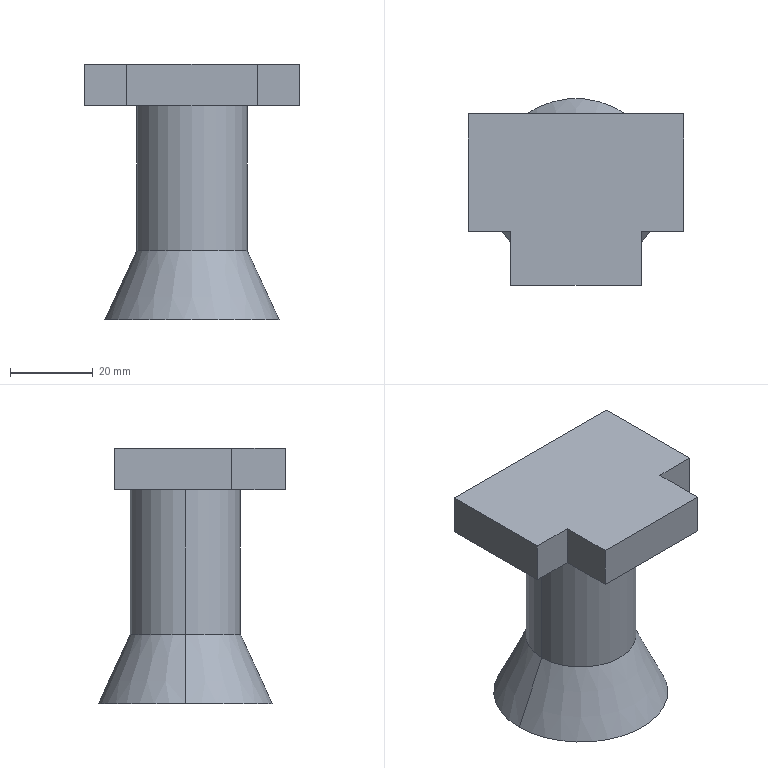Part | SolidWorks | features Extrusion 1, ICE 1, Revolution 1 | 1 solid | 15 faces | box 51.992 x 45.152 x 61.712 mm | volume 54023 mm3 | plane 11 | cone 2 | cylinder 2 | commonest cylinder face diameters 26.601 x2
STEP:
#1=CARTESIAN_POINT('',(-13.301,24.131,-45.));
#2=VERTEX_POINT('',#1);
#3=CARTESIAN_POINT('',(13.301,24.131,-45.));
#4=VERTEX_POINT('',#3);
#5=CARTESIAN_POINT('',(0.,24.131,-45.));
#6=DIRECTION('',(0.,0.,-1.));
#7=DIRECTION('',(-1.,0.,0.));
#8=AXIS2_PLACEMENT_3D('',#5,#6,#7);
#9=CIRCLE('',#8,13.301);
#10=EDGE_CURVE('',#2,#4,#9,.T.);
#11=ORIENTED_EDGE('',*,*,#10,.T.);
#12=CARTESIAN_POINT('',(21.021,24.131,-61.712));
#13=VERTEX_POINT('',#12);
#14=CARTESIAN_POINT('',(21.021,24.131,-61.712));
#15=DIRECTION('',(0.4194,0.,-0.9078));
#16=VECTOR('',#15,1000.);
#17=LINE('',#14,#16);
#18=EDGE_CURVE('',#4,#13,#17,.T.);
#19=ORIENTED_EDGE('',*,*,#18,.T.);
#20=CARTESIAN_POINT('',(-21.021,24.131,-61.712));
#21=VERTEX_POINT('',#20);
#22=CARTESIAN_POINT('',(0.,24.131,-61.712));
#23=DIRECTION('',(0.,0.,1.));
#24=DIRECTION('',(1.,0.,0.));
#25=AXIS2_PLACEMENT_3D('',#22,#23,#24);
#26=CIRCLE('',#25,21.021);
#27=EDGE_CURVE('',#13,#21,#26,.T.);
#28=ORIENTED_EDGE('',*,*,#27,.T.);
#29=CARTESIAN_POINT('',(-21.021,24.131,-61.712));
#30=DIRECTION('',(-0.4194,0.,-0.9078));
#31=VECTOR('',#30,1000.);
#32=LINE('',#29,#31);
#33=EDGE_CURVE('',#2,#21,#32,.T.);
#34=ORIENTED_EDGE('',*,*,#33,.F.);
#35=EDGE_LOOP('',(#11,#19,#28,#34));
#36=FACE_OUTER_BOUND('',#35,.T.);
#37=CARTESIAN_POINT('',(0.,24.131,-61.712));
#38=DIRECTION('',(0.,0.,-1.));
#39=DIRECTION('',(-1.,0.,0.));
#40=AXIS2_PLACEMENT_3D('',#37,#38,#39);
#41=CONICAL_SURFACE('',#40,21.021,0.4328);
#42=ADVANCED_FACE('',(#36),#41,.T.);
#43=ORIENTED_EDGE('',*,*,#10,.F.);
#44=CARTESIAN_POINT('',(-13.301,24.131,-10.));
#45=VERTEX_POINT('',#44);
#46=CARTESIAN_POINT('',(-13.301,24.131,-45.));
#47=DIRECTION('',(0.,0.,1.));
#48=VECTOR('',#47,1000.);
#49=LINE('',#46,#48);
#50=EDGE_CURVE('',#2,#45,#49,.T.);
#51=ORIENTED_EDGE('',*,*,#50,.T.);
#52=CARTESIAN_POINT('',(13.301,24.131,-10.));
#53=VERTEX_POINT('',#52);
#54=CARTESIAN_POINT('',(0.,24.131,-10.));
#55=DIRECTION('',(0.,0.,-1.));
#56=DIRECTION('',(1.,0.,0.));
#57=AXIS2_PLACEMENT_3D('',#54,#55,#56);
#58=CIRCLE('',#57,13.301);
#59=EDGE_CURVE('',#45,#53,#58,.T.);
#60=ORIENTED_EDGE('',*,*,#59,.T.);
#61=CARTESIAN_POINT('',(13.301,24.131,-45.));
#62=DIRECTION('',(0.,0.,1.));
#63=VECTOR('',#62,1000.);
#64=LINE('',#61,#63);
#65=EDGE_CURVE('',#4,#53,#64,.T.);
#66=ORIENTED_EDGE('',*,*,#65,.F.);
#67=EDGE_LOOP('',(#43,#51,#60,#66));
#68=FACE_OUTER_BOUND('',#67,.T.);
#69=CARTESIAN_POINT('',(0.,24.131,-45.));
#70=DIRECTION('',(0.,0.,1.));
#71=DIRECTION('',(1.,0.,0.));
#72=AXIS2_PLACEMENT_3D('',#69,#70,#71);
#73=CYLINDRICAL_SURFACE('',#72,13.301);
#74=ADVANCED_FACE('',(#68),#73,.T.);
#75=CARTESIAN_POINT('',(15.792,12.933,0.));
#76=VERTEX_POINT('',#75);
#77=CARTESIAN_POINT('',(25.996,12.933,0.));
#78=VERTEX_POINT('',#77);
#79=CARTESIAN_POINT('',(15.792,12.933,0.));
#80=DIRECTION('',(1.,0.,0.));
#81=VECTOR('',#80,1000.);
#82=LINE('',#79,#81);
#83=EDGE_CURVE('',#76,#78,#82,.T.);
#84=ORIENTED_EDGE('',*,*,#83,.F.);
#85=CARTESIAN_POINT('',(15.792,12.933,-10.));
#86=VERTEX_POINT('',#85);
#87=CARTESIAN_POINT('',(15.792,12.933,-10.));
#88=DIRECTION('',(0.,0.,1.));
#89=VECTOR('',#88,1000.);
#90=LINE('',#87,#89);
#91=EDGE_CURVE('',#86,#76,#90,.T.);
#92=ORIENTED_EDGE('',*,*,#91,.F.);
#93=CARTESIAN_POINT('',(25.996,12.933,-10.));
#94=VERTEX_POINT('',#93);
#95=CARTESIAN_POINT('',(15.792,12.933,-10.));
#96=DIRECTION('',(1.,0.,0.));
#97=VECTOR('',#96,1000.);
#98=LINE('',#95,#97);
#99=EDGE_CURVE('',#86,#94,#98,.T.);
#100=ORIENTED_EDGE('',*,*,#99,.T.);
#101=CARTESIAN_POINT('',(25.996,12.933,-10.));
#102=DIRECTION('',(0.,0.,1.));
#103=VECTOR('',#102,1000.);
#104=LINE('',#101,#103);
#105=EDGE_CURVE('',#94,#78,#104,.T.);
#106=ORIENTED_EDGE('',*,*,#105,.T.);
#107=EDGE_LOOP('',(#84,#92,#100,#106));
#108=FACE_OUTER_BOUND('',#107,.T.);
#109=CARTESIAN_POINT('',(15.792,12.933,-10.));
#110=DIRECTION('',(0.,-1.,0.));
#111=DIRECTION('',(0.,0.,-1.));
#112=AXIS2_PLACEMENT_3D('',#109,#110,#111);
#113=PLANE('',#112);
#114=ADVANCED_FACE('',(#108),#113,.T.);
#115=CARTESIAN_POINT('',(15.792,0.,0.));
#116=VERTEX_POINT('',#115);
#117=CARTESIAN_POINT('',(15.792,0.,0.));
#118=DIRECTION('',(0.,1.,0.));
#119=VECTOR('',#118,1000.);
#120=LINE('',#117,#119);
#121=EDGE_CURVE('',#116,#76,#120,.T.);
#122=ORIENTED_EDGE('',*,*,#121,.F.);
#123=CARTESIAN_POINT('',(15.792,0.,-10.));
#124=VERTEX_POINT('',#123);
#125=CARTESIAN_POINT('',(15.792,0.,-10.));
#126=DIRECTION('',(0.,0.,1.));
#127=VECTOR('',#126,1000.);
#128=LINE('',#125,#127);
#129=EDGE_CURVE('',#124,#116,#128,.T.);
#130=ORIENTED_EDGE('',*,*,#129,.F.);
#131=CARTESIAN_POINT('',(15.792,0.,-10.));
#132=DIRECTION('',(0.,1.,0.));
#133=VECTOR('',#132,1000.);
#134=LINE('',#131,#133);
#135=EDGE_CURVE('',#124,#86,#134,.T.);
#136=ORIENTED_EDGE('',*,*,#135,.T.);
#137=ORIENTED_EDGE('',*,*,#91,.T.);
#138=EDGE_LOOP('',(#122,#130,#136,#137));
#139=FACE_OUTER_BOUND('',#138,.T.);
#140=CARTESIAN_POINT('',(15.792,0.,-10.));
#141=DIRECTION('',(1.,0.,0.));
#142=DIRECTION('',(0.,0.,-1.));
#143=AXIS2_PLACEMENT_3D('',#140,#141,#142);
#144=PLANE('',#143);
#145=ADVANCED_FACE('',(#139),#144,.T.);
#146=CARTESIAN_POINT('',(-15.792,0.,0.));
#147=VERTEX_POINT('',#146);
#148=CARTESIAN_POINT('',(15.792,0.,0.));
#149=DIRECTION('',(1.,0.,0.));
#150=VECTOR('',#149,1000.);
#151=LINE('',#148,#150);
#152=EDGE_CURVE('',#147,#116,#151,.T.);
#153=ORIENTED_EDGE('',*,*,#152,.F.);
#154=CARTESIAN_POINT('',(-15.792,0.,-10.));
#155=VERTEX_POINT('',#154);
#156=CARTESIAN_POINT('',(-15.792,0.,-10.));
#157=DIRECTION('',(0.,0.,1.));
#158=VECTOR('',#157,1000.);
#159=LINE('',#156,#158);
#160=EDGE_CURVE('',#155,#147,#159,.T.);
#161=ORIENTED_EDGE('',*,*,#160,.F.);
#162=CARTESIAN_POINT('',(15.792,0.,-10.));
#163=DIRECTION('',(1.,0.,0.));
#164=VECTOR('',#163,1000.);
#165=LINE('',#162,#164);
#166=EDGE_CURVE('',#155,#124,#165,.T.);
#167=ORIENTED_EDGE('',*,*,#166,.T.);
#168=ORIENTED_EDGE('',*,*,#129,.T.);
#169=EDGE_LOOP('',(#153,#161,#167,#168));
#170=FACE_OUTER_BOUND('',#169,.T.);
#171=CARTESIAN_POINT('',(15.792,0.,-10.));
#172=DIRECTION('',(0.,-1.,0.));
#173=DIRECTION('',(0.,0.,-1.));
#174=AXIS2_PLACEMENT_3D('',#171,#172,#173);
#175=PLANE('',#174);
#176=ADVANCED_FACE('',(#170),#175,.T.);
#177=CARTESIAN_POINT('',(-15.792,12.933,0.));
#178=VERTEX_POINT('',#177);
#179=CARTESIAN_POINT('',(-15.792,0.,0.));
#180=DIRECTION('',(0.,-1.,0.));
#181=VECTOR('',#180,1000.);
#182=LINE('',#179,#181);
#183=EDGE_CURVE('',#178,#147,#182,.T.);
#184=ORIENTED_EDGE('',*,*,#183,.F.);
#185=CARTESIAN_POINT('',(-15.792,12.933,-10.));
#186=VERTEX_POINT('',#185);
#187=CARTESIAN_POINT('',(-15.792,12.933,-10.));
#188=DIRECTION('',(0.,0.,1.));
#189=VECTOR('',#188,1000.);
#190=LINE('',#187,#189);
#191=EDGE_CURVE('',#186,#178,#190,.T.);
#192=ORIENTED_EDGE('',*,*,#191,.F.);
#193=CARTESIAN_POINT('',(-15.792,0.,-10.));
#194=DIRECTION('',(0.,-1.,0.));
#195=VECTOR('',#194,1000.);
#196=LINE('',#193,#195);
#197=EDGE_CURVE('',#186,#155,#196,.T.);
#198=ORIENTED_EDGE('',*,*,#197,.T.);
#199=ORIENTED_EDGE('',*,*,#160,.T.);
#200=EDGE_LOOP('',(#184,#192,#198,#199));
#201=FACE_OUTER_BOUND('',#200,.T.);
#202=CARTESIAN_POINT('',(-15.792,0.,-10.));
#203=DIRECTION('',(-1.,0.,0.));
#204=DIRECTION('',(0.,0.,1.));
#205=AXIS2_PLACEMENT_3D('',#202,#203,#204);
#206=PLANE('',#205);
#207=ADVANCED_FACE('',(#201),#206,.T.);
#208=CARTESIAN_POINT('',(-25.996,12.933,0.));
#209=VERTEX_POINT('',#208);
#210=CARTESIAN_POINT('',(-15.792,12.933,0.));
#211=DIRECTION('',(1.,0.,0.));
#212=VECTOR('',#211,1000.);
#213=LINE('',#210,#212);
#214=EDGE_CURVE('',#209,#178,#213,.T.);
#215=ORIENTED_EDGE('',*,*,#214,.F.);
#216=CARTESIAN_POINT('',(-25.996,12.933,-10.));
#217=VERTEX_POINT('',#216);
#218=CARTESIAN_POINT('',(-25.996,12.933,-10.));
#219=DIRECTION('',(0.,0.,1.));
#220=VECTOR('',#219,1000.);
#221=LINE('',#218,#220);
#222=EDGE_CURVE('',#217,#209,#221,.T.);
#223=ORIENTED_EDGE('',*,*,#222,.F.);
#224=CARTESIAN_POINT('',(-15.792,12.933,-10.));
#225=DIRECTION('',(1.,0.,0.));
#226=VECTOR('',#225,1000.);
#227=LINE('',#224,#226);
#228=EDGE_CURVE('',#217,#186,#227,.T.);
#229=ORIENTED_EDGE('',*,*,#228,.T.);
#230=ORIENTED_EDGE('',*,*,#191,.T.);
#231=EDGE_LOOP('',(#215,#223,#229,#230));
#232=FACE_OUTER_BOUND('',#231,.T.);
#233=CARTESIAN_POINT('',(-15.792,12.933,-10.));
#234=DIRECTION('',(0.,-1.,0.));
#235=DIRECTION('',(0.,0.,-1.));
#236=AXIS2_PLACEMENT_3D('',#233,#234,#235);
#237=PLANE('',#236);
#238=ADVANCED_FACE('',(#232),#237,.T.);
#239=CARTESIAN_POINT('',(-25.996,41.33,0.));
#240=VERTEX_POINT('',#239);
#241=CARTESIAN_POINT('',(-25.996,12.933,0.));
#242=DIRECTION('',(0.,-1.,0.));
#243=VECTOR('',#242,1000.);
#244=LINE('',#241,#243);
#245=EDGE_CURVE('',#240,#209,#244,.T.);
#246=ORIENTED_EDGE('',*,*,#245,.F.);
#247=CARTESIAN_POINT('',(-25.996,41.33,-10.));
#248=VERTEX_POINT('',#247);
#249=CARTESIAN_POINT('',(-25.996,41.33,-10.));
#250=DIRECTION('',(0.,0.,1.));
#251=VECTOR('',#250,1000.);
#252=LINE('',#249,#251);
#253=EDGE_CURVE('',#248,#240,#252,.T.);
#254=ORIENTED_EDGE('',*,*,#253,.F.);
#255=CARTESIAN_POINT('',(-25.996,12.933,-10.));
#256=DIRECTION('',(0.,-1.,0.));
#257=VECTOR('',#256,1000.);
#258=LINE('',#255,#257);
#259=EDGE_CURVE('',#248,#217,#258,.T.);
#260=ORIENTED_EDGE('',*,*,#259,.T.);
#261=ORIENTED_EDGE('',*,*,#222,.T.);
#262=EDGE_LOOP('',(#246,#254,#260,#261));
#263=FACE_OUTER_BOUND('',#262,.T.);
#264=CARTESIAN_POINT('',(-25.996,12.933,-10.));
#265=DIRECTION('',(-1.,0.,0.));
#266=DIRECTION('',(0.,0.,1.));
#267=AXIS2_PLACEMENT_3D('',#264,#265,#266);
#268=PLANE('',#267);
#269=ADVANCED_FACE('',(#263),#268,.T.);
#270=CARTESIAN_POINT('',(25.996,41.33,0.));
#271=VERTEX_POINT('',#270);
#272=CARTESIAN_POINT('',(-25.996,41.33,0.));
#273=DIRECTION('',(-1.,0.,0.));
#274=VECTOR('',#273,1000.);
#275=LINE('',#272,#274);
#276=EDGE_CURVE('',#271,#240,#275,.T.);
#277=ORIENTED_EDGE('',*,*,#276,.F.);
#278=CARTESIAN_POINT('',(25.996,41.33,-10.));
#279=VERTEX_POINT('',#278);
#280=CARTESIAN_POINT('',(25.996,41.33,-10.));
#281=DIRECTION('',(0.,0.,1.));
#282=VECTOR('',#281,1000.);
#283=LINE('',#280,#282);
#284=EDGE_CURVE('',#279,#271,#283,.T.);
#285=ORIENTED_EDGE('',*,*,#284,.F.);
#286=CARTESIAN_POINT('',(-25.996,41.33,-10.));
#287=DIRECTION('',(-1.,0.,0.));
#288=VECTOR('',#287,1000.);
#289=LINE('',#286,#288);
#290=EDGE_CURVE('',#279,#248,#289,.T.);
#291=ORIENTED_EDGE('',*,*,#290,.T.);
#292=ORIENTED_EDGE('',*,*,#253,.T.);
#293=EDGE_LOOP('',(#277,#285,#291,#292));
#294=FACE_OUTER_BOUND('',#293,.T.);
#295=CARTESIAN_POINT('',(-25.996,41.33,-10.));
#296=DIRECTION('',(0.,1.,0.));
#297=DIRECTION('',(0.,0.,1.));
#298=AXIS2_PLACEMENT_3D('',#295,#296,#297);
#299=PLANE('',#298);
#300=ADVANCED_FACE('',(#294),#299,.T.);
#301=CARTESIAN_POINT('',(25.996,12.933,0.));
#302=DIRECTION('',(0.,1.,0.));
#303=VECTOR('',#302,1000.);
#304=LINE('',#301,#303);
#305=EDGE_CURVE('',#78,#271,#304,.T.);
#306=ORIENTED_EDGE('',*,*,#305,.F.);
#307=ORIENTED_EDGE('',*,*,#105,.F.);
#308=CARTESIAN_POINT('',(25.996,12.933,-10.));
#309=DIRECTION('',(0.,1.,0.));
#310=VECTOR('',#309,1000.);
#311=LINE('',#308,#310);
#312=EDGE_CURVE('',#94,#279,#311,.T.);
#313=ORIENTED_EDGE('',*,*,#312,.T.);
#314=ORIENTED_EDGE('',*,*,#284,.T.);
#315=EDGE_LOOP('',(#306,#307,#313,#314));
#316=FACE_OUTER_BOUND('',#315,.T.);
#317=CARTESIAN_POINT('',(25.996,12.933,-10.));
#318=DIRECTION('',(1.,0.,0.));
#319=DIRECTION('',(0.,0.,-1.));
#320=AXIS2_PLACEMENT_3D('',#317,#318,#319);
#321=PLANE('',#320);
#322=ADVANCED_FACE('',(#316),#321,.T.);
#323=CARTESIAN_POINT('',(0.,24.131,-10.));
#324=DIRECTION('',(0.,0.,-1.));
#325=DIRECTION('',(1.,0.,0.));
#326=AXIS2_PLACEMENT_3D('',#323,#324,#325);
#327=CIRCLE('',#326,13.301);
#328=EDGE_CURVE('',#53,#45,#327,.T.);
#329=ORIENTED_EDGE('',*,*,#328,.F.);
#330=ORIENTED_EDGE('',*,*,#59,.F.);
#331=EDGE_LOOP('',(#329,#330));
#332=FACE_BOUND('',#331,.T.);
#333=ORIENTED_EDGE('',*,*,#99,.F.);
#334=ORIENTED_EDGE('',*,*,#135,.F.);
#335=ORIENTED_EDGE('',*,*,#166,.F.);
#336=ORIENTED_EDGE('',*,*,#197,.F.);
#337=ORIENTED_EDGE('',*,*,#228,.F.);
#338=ORIENTED_EDGE('',*,*,#259,.F.);
#339=ORIENTED_EDGE('',*,*,#290,.F.);
#340=ORIENTED_EDGE('',*,*,#312,.F.);
#341=EDGE_LOOP('',(#333,#334,#335,#336,#337,#338,#339,#340));
#342=FACE_OUTER_BOUND('',#341,.T.);
#343=CARTESIAN_POINT('',(0.,0.,-10.));
#344=DIRECTION('',(0.,0.,1.));
#345=DIRECTION('',(1.,0.,0.));
#346=AXIS2_PLACEMENT_3D('',#343,#344,#345);
#347=PLANE('',#346);
#348=ADVANCED_FACE('',(#332,#342),#347,.F.);
#349=ORIENTED_EDGE('',*,*,#83,.T.);
#350=ORIENTED_EDGE('',*,*,#305,.T.);
#351=ORIENTED_EDGE('',*,*,#276,.T.);
#352=ORIENTED_EDGE('',*,*,#245,.T.);
#353=ORIENTED_EDGE('',*,*,#214,.T.);
#354=ORIENTED_EDGE('',*,*,#183,.T.);
#355=ORIENTED_EDGE('',*,*,#152,.T.);
#356=ORIENTED_EDGE('',*,*,#121,.T.);
#357=EDGE_LOOP('',(#349,#350,#351,#352,#353,#354,#355,#356));
#358=FACE_OUTER_BOUND('',#357,.T.);
#359=CARTESIAN_POINT('',(0.,0.,0.));
#360=DIRECTION('',(0.,0.,1.));
#361=DIRECTION('',(1.,0.,0.));
#362=AXIS2_PLACEMENT_3D('',#359,#360,#361);
#363=PLANE('',#362);
#364=ADVANCED_FACE('',(#358),#363,.T.);
#365=ORIENTED_EDGE('',*,*,#50,.F.);
#366=CARTESIAN_POINT('',(0.,24.131,-45.));
#367=DIRECTION('',(0.,0.,-1.));
#368=DIRECTION('',(-1.,0.,0.));
#369=AXIS2_PLACEMENT_3D('',#366,#367,#368);
#370=CIRCLE('',#369,13.301);
#371=EDGE_CURVE('',#4,#2,#370,.T.);
#372=ORIENTED_EDGE('',*,*,#371,.F.);
#373=ORIENTED_EDGE('',*,*,#65,.T.);
#374=ORIENTED_EDGE('',*,*,#328,.T.);
#375=EDGE_LOOP('',(#365,#372,#373,#374));
#376=FACE_OUTER_BOUND('',#375,.T.);
#377=CARTESIAN_POINT('',(0.,24.131,-45.));
#378=DIRECTION('',(0.,0.,1.));
#379=DIRECTION('',(1.,0.,0.));
#380=AXIS2_PLACEMENT_3D('',#377,#378,#379);
#381=CYLINDRICAL_SURFACE('',#380,13.301);
#382=ADVANCED_FACE('',(#376),#381,.T.);
#383=CARTESIAN_POINT('',(0.,24.131,-61.712));
#384=DIRECTION('',(0.,0.,1.));
#385=DIRECTION('',(1.,0.,0.));
#386=AXIS2_PLACEMENT_3D('',#383,#384,#385);
#387=CIRCLE('',#386,21.021);
#388=EDGE_CURVE('',#21,#13,#387,.T.);
#389=ORIENTED_EDGE('',*,*,#388,.F.);
#390=ORIENTED_EDGE('',*,*,#27,.F.);
#391=EDGE_LOOP('',(#389,#390));
#392=FACE_OUTER_BOUND('',#391,.T.);
#393=CARTESIAN_POINT('',(0.,45.152,-61.712));
#394=DIRECTION('',(0.,0.,1.));
#395=DIRECTION('',(1.,0.,0.));
#396=AXIS2_PLACEMENT_3D('',#393,#394,#395);
#397=PLANE('',#396);
#398=ADVANCED_FACE('',(#392),#397,.F.);
#399=ORIENTED_EDGE('',*,*,#18,.F.);
#400=ORIENTED_EDGE('',*,*,#371,.T.);
#401=ORIENTED_EDGE('',*,*,#33,.T.);
#402=ORIENTED_EDGE('',*,*,#388,.T.);
#403=EDGE_LOOP('',(#399,#400,#401,#402));
#404=FACE_OUTER_BOUND('',#403,.T.);
#405=CARTESIAN_POINT('',(0.,24.131,-61.712));
#406=DIRECTION('',(0.,0.,-1.));
#407=DIRECTION('',(-1.,0.,0.));
#408=AXIS2_PLACEMENT_3D('',#405,#406,#407);
#409=CONICAL_SURFACE('',#408,21.021,0.4328);
#410=ADVANCED_FACE('',(#404),#409,.T.);
#411=CLOSED_SHELL('',(#42,#74,#114,#145,#176,#207,#238,#269,#300,#322,#348,#364,#382,#398,#410));
#412=MANIFOLD_SOLID_BREP('',#411);
#413=CARTESIAN_POINT('',(0.,0.,0.));
#414=DIRECTION('',(0.,0.,1.));
#415=DIRECTION('',(1.,0.,0.));
#416=AXIS2_PLACEMENT_3D('',#413,#414,#415);
#417=(LENGTH_UNIT()NAMED_UNIT(*)SI_UNIT(.MILLI.,.METRE.));
#418=UNCERTAINTY_MEASURE_WITH_UNIT(LENGTH_MEASURE(0.00001),#417,'','');
#419=(NAMED_UNIT(*)PLANE_ANGLE_UNIT()SI_UNIT($,.RADIAN.));
#420=(NAMED_UNIT(*)SI_UNIT($,.STERADIAN.)SOLID_ANGLE_UNIT());
#421=(GEOMETRIC_REPRESENTATION_CONTEXT(3)GLOBAL_UNCERTAINTY_ASSIGNED_CONTEXT((#418))GLOBAL_UNIT_ASSIGNED_CONTEXT((#417,#419,#420))REPRESENTATION_CONTEXT('',''));
#422=ADVANCED_BREP_SHAPE_REPRESENTATION('',(#412,#416),#421);